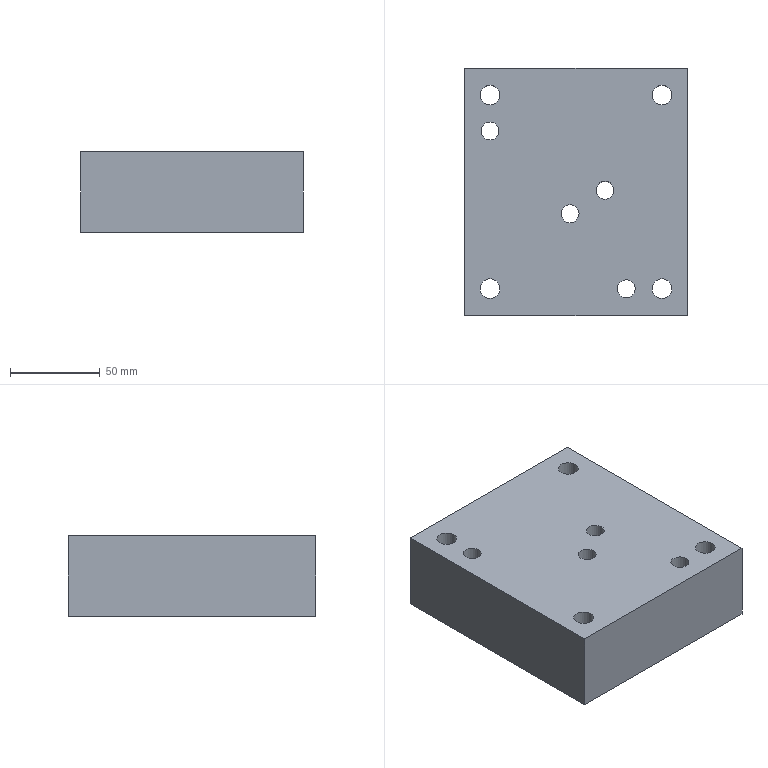Part | NX | features solid 2 | 1 solid | 32 faces | box 124 x 138 x 45 mm | volume 721952 mm3 | cylinder 17 | plane 12 | cone 3 | commonest cylinder face diameters 10 x4 11 x4 17 x4 8.5 x3 12 x2
STEP:
#1=CARTESIAN_POINT('',(391.63,-102.164,63.));
#2=VERTEX_POINT('',#1);
#3=CARTESIAN_POINT('',(397.13,-102.164,63.));
#4=DIRECTION('',(0.,0.,1.));
#5=DIRECTION('',(-1.,0.,0.));
#6=AXIS2_PLACEMENT_3D('',#3,#4,#5);
#7=CIRCLE('',#6,5.5);
#8=EDGE_CURVE('',#2,#2,#7,.T.);
#9=ORIENTED_EDGE('',*,*,#8,.T.);
#10=EDGE_LOOP('',(#9));
#11=FACE_BOUND('',#10,.T.);
#12=CARTESIAN_POINT('',(388.63,-102.164,63.));
#13=VERTEX_POINT('',#12);
#14=CARTESIAN_POINT('',(397.13,-102.164,63.));
#15=DIRECTION('',(0.,0.,1.));
#16=DIRECTION('',(-1.,0.,0.));
#17=AXIS2_PLACEMENT_3D('',#14,#15,#16);
#18=CIRCLE('',#17,8.5);
#19=EDGE_CURVE('',#13,#13,#18,.T.);
#20=ORIENTED_EDGE('',*,*,#19,.F.);
#21=EDGE_LOOP('',(#20));
#22=FACE_BOUND('',#21,.T.);
#23=CARTESIAN_POINT('',(188.,0.,63.));
#24=DIRECTION('',(0.,0.,-1.));
#25=DIRECTION('',(-1.,0.,0.));
#26=AXIS2_PLACEMENT_3D('',#23,#24,#25);
#27=PLANE('',#26);
#28=ADVANCED_FACE('',(#11,#22),#27,.T.);
#29=CARTESIAN_POINT('',(498.63,-102.164,63.));
#30=VERTEX_POINT('',#29);
#31=CARTESIAN_POINT('',(493.13,-102.164,63.));
#32=DIRECTION('',(0.,0.,-1.));
#33=DIRECTION('',(1.,0.,0.));
#34=AXIS2_PLACEMENT_3D('',#31,#32,#33);
#35=CIRCLE('',#34,5.5);
#36=EDGE_CURVE('',#30,#30,#35,.F.);
#37=ORIENTED_EDGE('',*,*,#36,.T.);
#38=EDGE_LOOP('',(#37));
#39=FACE_BOUND('',#38,.T.);
#40=CARTESIAN_POINT('',(501.63,-102.164,63.));
#41=VERTEX_POINT('',#40);
#42=CARTESIAN_POINT('',(493.13,-102.164,63.));
#43=DIRECTION('',(0.,0.,-1.));
#44=DIRECTION('',(1.,0.,0.));
#45=AXIS2_PLACEMENT_3D('',#42,#43,#44);
#46=CIRCLE('',#45,8.5);
#47=EDGE_CURVE('',#41,#41,#46,.F.);
#48=ORIENTED_EDGE('',*,*,#47,.F.);
#49=EDGE_LOOP('',(#48));
#50=FACE_BOUND('',#49,.T.);
#51=CARTESIAN_POINT('',(702.259,0.,63.));
#52=DIRECTION('',(0.,0.,-1.));
#53=DIRECTION('',(1.,0.,0.));
#54=AXIS2_PLACEMENT_3D('',#51,#52,#53);
#55=PLANE('',#54);
#56=ADVANCED_FACE('',(#39,#50),#55,.T.);
#57=CARTESIAN_POINT('',(498.63,-210.164,63.));
#58=VERTEX_POINT('',#57);
#59=CARTESIAN_POINT('',(493.13,-210.164,63.));
#60=DIRECTION('',(0.,0.,1.));
#61=DIRECTION('',(1.,0.,0.));
#62=AXIS2_PLACEMENT_3D('',#59,#60,#61);
#63=CIRCLE('',#62,5.5);
#64=EDGE_CURVE('',#58,#58,#63,.T.);
#65=ORIENTED_EDGE('',*,*,#64,.T.);
#66=EDGE_LOOP('',(#65));
#67=FACE_BOUND('',#66,.T.);
#68=CARTESIAN_POINT('',(501.63,-210.164,63.));
#69=VERTEX_POINT('',#68);
#70=CARTESIAN_POINT('',(493.13,-210.164,63.));
#71=DIRECTION('',(0.,0.,1.));
#72=DIRECTION('',(1.,0.,0.));
#73=AXIS2_PLACEMENT_3D('',#70,#71,#72);
#74=CIRCLE('',#73,8.5);
#75=EDGE_CURVE('',#69,#69,#74,.T.);
#76=ORIENTED_EDGE('',*,*,#75,.F.);
#77=EDGE_LOOP('',(#76));
#78=FACE_BOUND('',#77,.T.);
#79=CARTESIAN_POINT('',(702.259,-312.328,63.));
#80=DIRECTION('',(0.,0.,-1.));
#81=DIRECTION('',(1.,0.,0.));
#82=AXIS2_PLACEMENT_3D('',#79,#80,#81);
#83=PLANE('',#82);
#84=ADVANCED_FACE('',(#67,#78),#83,.T.);
#85=CARTESIAN_POINT('',(391.63,-210.164,63.));
#86=VERTEX_POINT('',#85);
#87=CARTESIAN_POINT('',(397.13,-210.164,63.));
#88=DIRECTION('',(0.,0.,-1.));
#89=DIRECTION('',(-1.,0.,0.));
#90=AXIS2_PLACEMENT_3D('',#87,#88,#89);
#91=CIRCLE('',#90,5.5);
#92=EDGE_CURVE('',#86,#86,#91,.F.);
#93=ORIENTED_EDGE('',*,*,#92,.T.);
#94=EDGE_LOOP('',(#93));
#95=FACE_BOUND('',#94,.T.);
#96=CARTESIAN_POINT('',(388.63,-210.164,63.));
#97=VERTEX_POINT('',#96);
#98=CARTESIAN_POINT('',(397.13,-210.164,63.));
#99=DIRECTION('',(0.,0.,-1.));
#100=DIRECTION('',(-1.,0.,0.));
#101=AXIS2_PLACEMENT_3D('',#98,#99,#100);
#102=CIRCLE('',#101,8.5);
#103=EDGE_CURVE('',#97,#97,#102,.F.);
#104=ORIENTED_EDGE('',*,*,#103,.F.);
#105=EDGE_LOOP('',(#104));
#106=FACE_BOUND('',#105,.T.);
#107=CARTESIAN_POINT('',(188.,-312.328,63.));
#108=DIRECTION('',(0.,0.,-1.));
#109=DIRECTION('',(-1.,0.,0.));
#110=AXIS2_PLACEMENT_3D('',#107,#108,#109);
#111=PLANE('',#110);
#112=ADVANCED_FACE('',(#95,#106),#111,.T.);
#113=CARTESIAN_POINT('',(402.13,-122.164,58.));
#114=VERTEX_POINT('',#113);
#115=CARTESIAN_POINT('',(397.13,-122.164,58.));
#116=DIRECTION('',(0.,0.,-1.));
#117=DIRECTION('',(1.,0.,0.));
#118=AXIS2_PLACEMENT_3D('',#115,#116,#117);
#119=CIRCLE('',#118,5.);
#120=EDGE_CURVE('',#114,#114,#119,.F.);
#121=ORIENTED_EDGE('',*,*,#120,.T.);
#122=EDGE_LOOP('',(#121));
#123=FACE_BOUND('',#122,.T.);
#124=CARTESIAN_POINT('',(403.13,-122.164,58.));
#125=VERTEX_POINT('',#124);
#126=CARTESIAN_POINT('',(397.13,-122.164,58.));
#127=DIRECTION('',(0.,0.,-1.));
#128=DIRECTION('',(1.,0.,0.));
#129=AXIS2_PLACEMENT_3D('',#126,#127,#128);
#130=CIRCLE('',#129,6.);
#131=EDGE_CURVE('',#125,#125,#130,.F.);
#132=ORIENTED_EDGE('',*,*,#131,.F.);
#133=EDGE_LOOP('',(#132));
#134=FACE_BOUND('',#133,.T.);
#135=CARTESIAN_POINT('',(397.575,-126.335,58.));
#136=DIRECTION('',(0.,0.,1.));
#137=DIRECTION('',(1.,0.,0.));
#138=AXIS2_PLACEMENT_3D('',#135,#136,#137);
#139=PLANE('',#138);
#140=ADVANCED_FACE('',(#123,#134),#139,.F.);
#141=CARTESIAN_POINT('',(402.13,-122.164,88.));
#142=VERTEX_POINT('',#141);
#143=CARTESIAN_POINT('',(397.13,-122.164,88.));
#144=DIRECTION('',(0.,0.,-1.));
#145=DIRECTION('',(1.,0.,0.));
#146=AXIS2_PLACEMENT_3D('',#143,#144,#145);
#147=CIRCLE('',#146,5.);
#148=EDGE_CURVE('',#142,#142,#147,.F.);
#149=ORIENTED_EDGE('',*,*,#148,.T.);
#150=EDGE_LOOP('',(#149));
#151=FACE_BOUND('',#150,.T.);
#152=ORIENTED_EDGE('',*,*,#120,.F.);
#153=EDGE_LOOP('',(#152));
#154=FACE_BOUND('',#153,.T.);
#155=CARTESIAN_POINT('',(397.13,-122.164,78.));
#156=DIRECTION('',(0.,0.,1.));
#157=DIRECTION('',(1.,0.,0.));
#158=AXIS2_PLACEMENT_3D('',#155,#156,#157);
#159=CYLINDRICAL_SURFACE('',#158,5.);
#160=ADVANCED_FACE('',(#151,#154),#159,.F.);
#161=CARTESIAN_POINT('',(402.63,-210.164,88.));
#162=VERTEX_POINT('',#161);
#163=CARTESIAN_POINT('',(397.13,-210.164,88.));
#164=DIRECTION('',(0.,0.,1.));
#165=DIRECTION('',(1.,0.,0.));
#166=AXIS2_PLACEMENT_3D('',#163,#164,#165);
#167=CIRCLE('',#166,5.5);
#168=EDGE_CURVE('',#162,#162,#167,.T.);
#169=ORIENTED_EDGE('',*,*,#168,.T.);
#170=EDGE_LOOP('',(#169));
#171=FACE_BOUND('',#170,.T.);
#172=ORIENTED_EDGE('',*,*,#92,.F.);
#173=EDGE_LOOP('',(#172));
#174=FACE_BOUND('',#173,.T.);
#175=CARTESIAN_POINT('',(397.13,-210.164,78.));
#176=DIRECTION('',(0.,0.,1.));
#177=DIRECTION('',(1.,0.,0.));
#178=AXIS2_PLACEMENT_3D('',#175,#176,#177);
#179=CYLINDRICAL_SURFACE('',#178,5.5);
#180=ADVANCED_FACE('',(#171,#174),#179,.F.);
#181=CARTESIAN_POINT('',(487.63,-210.164,88.));
#182=VERTEX_POINT('',#181);
#183=CARTESIAN_POINT('',(493.13,-210.164,88.));
#184=DIRECTION('',(0.,0.,-1.));
#185=DIRECTION('',(-1.,0.,0.));
#186=AXIS2_PLACEMENT_3D('',#183,#184,#185);
#187=CIRCLE('',#186,5.5);
#188=EDGE_CURVE('',#182,#182,#187,.F.);
#189=ORIENTED_EDGE('',*,*,#188,.T.);
#190=EDGE_LOOP('',(#189));
#191=FACE_BOUND('',#190,.T.);
#192=ORIENTED_EDGE('',*,*,#64,.F.);
#193=EDGE_LOOP('',(#192));
#194=FACE_BOUND('',#193,.T.);
#195=CARTESIAN_POINT('',(493.13,-210.164,78.));
#196=DIRECTION('',(0.,0.,1.));
#197=DIRECTION('',(-1.,0.,0.));
#198=AXIS2_PLACEMENT_3D('',#195,#196,#197);
#199=CYLINDRICAL_SURFACE('',#198,5.5);
#200=ADVANCED_FACE('',(#191,#194),#199,.F.);
#201=CARTESIAN_POINT('',(487.63,-102.164,88.));
#202=VERTEX_POINT('',#201);
#203=CARTESIAN_POINT('',(493.13,-102.164,88.));
#204=DIRECTION('',(0.,0.,1.));
#205=DIRECTION('',(-1.,0.,0.));
#206=AXIS2_PLACEMENT_3D('',#203,#204,#205);
#207=CIRCLE('',#206,5.5);
#208=EDGE_CURVE('',#202,#202,#207,.T.);
#209=ORIENTED_EDGE('',*,*,#208,.T.);
#210=EDGE_LOOP('',(#209));
#211=FACE_BOUND('',#210,.T.);
#212=ORIENTED_EDGE('',*,*,#36,.F.);
#213=EDGE_LOOP('',(#212));
#214=FACE_BOUND('',#213,.T.);
#215=CARTESIAN_POINT('',(493.13,-102.164,78.));
#216=DIRECTION('',(0.,0.,1.));
#217=DIRECTION('',(-1.,0.,0.));
#218=AXIS2_PLACEMENT_3D('',#215,#216,#217);
#219=CYLINDRICAL_SURFACE('',#218,5.5);
#220=ADVANCED_FACE('',(#211,#214),#219,.F.);
#221=CARTESIAN_POINT('',(383.13,-225.164,43.));
#222=VERTEX_POINT('',#221);
#223=CARTESIAN_POINT('',(383.13,-225.164,88.));
#224=VERTEX_POINT('',#223);
#225=CARTESIAN_POINT('',(383.13,-225.164,62.));
#226=DIRECTION('',(0.,0.,1.));
#227=VECTOR('',#226,1000.);
#228=LINE('',#225,#227);
#229=EDGE_CURVE('',#222,#224,#228,.T.);
#230=ORIENTED_EDGE('',*,*,#229,.F.);
#231=CARTESIAN_POINT('',(507.13,-225.164,43.));
#232=VERTEX_POINT('',#231);
#233=CARTESIAN_POINT('',(445.13,-225.164,43.));
#234=DIRECTION('',(-1.,0.,0.));
#235=VECTOR('',#234,1000.);
#236=LINE('',#233,#235);
#237=EDGE_CURVE('',#232,#222,#236,.T.);
#238=ORIENTED_EDGE('',*,*,#237,.F.);
#239=CARTESIAN_POINT('',(507.13,-225.164,88.));
#240=VERTEX_POINT('',#239);
#241=CARTESIAN_POINT('',(507.13,-225.164,62.));
#242=DIRECTION('',(0.,0.,1.));
#243=VECTOR('',#242,1000.);
#244=LINE('',#241,#243);
#245=EDGE_CURVE('',#232,#240,#244,.T.);
#246=ORIENTED_EDGE('',*,*,#245,.T.);
#247=CARTESIAN_POINT('',(445.13,-225.164,88.));
#248=DIRECTION('',(1.,0.,0.));
#249=VECTOR('',#248,1000.);
#250=LINE('',#247,#249);
#251=EDGE_CURVE('',#224,#240,#250,.T.);
#252=ORIENTED_EDGE('',*,*,#251,.F.);
#253=EDGE_LOOP('',(#230,#238,#246,#252));
#254=FACE_BOUND('',#253,.T.);
#255=CARTESIAN_POINT('',(445.13,-225.164,62.));
#256=DIRECTION('',(0.,-1.,0.));
#257=DIRECTION('',(0.,0.,1.));
#258=AXIS2_PLACEMENT_3D('',#255,#256,#257);
#259=PLANE('',#258);
#260=ADVANCED_FACE('',(#254),#259,.T.);
#261=CARTESIAN_POINT('',(383.13,-87.164,43.));
#262=VERTEX_POINT('',#261);
#263=CARTESIAN_POINT('',(383.13,-87.164,88.));
#264=VERTEX_POINT('',#263);
#265=CARTESIAN_POINT('',(383.13,-87.164,62.));
#266=DIRECTION('',(0.,0.,1.));
#267=VECTOR('',#266,1000.);
#268=LINE('',#265,#267);
#269=EDGE_CURVE('',#262,#264,#268,.T.);
#270=ORIENTED_EDGE('',*,*,#269,.F.);
#271=CARTESIAN_POINT('',(383.13,-154.023,43.));
#272=DIRECTION('',(0.,1.,0.));
#273=VECTOR('',#272,1000.);
#274=LINE('',#271,#273);
#275=EDGE_CURVE('',#222,#262,#274,.T.);
#276=ORIENTED_EDGE('',*,*,#275,.F.);
#277=ORIENTED_EDGE('',*,*,#229,.T.);
#278=CARTESIAN_POINT('',(383.13,-154.023,88.));
#279=DIRECTION('',(0.,-1.,0.));
#280=VECTOR('',#279,1000.);
#281=LINE('',#278,#280);
#282=EDGE_CURVE('',#264,#224,#281,.T.);
#283=ORIENTED_EDGE('',*,*,#282,.F.);
#284=EDGE_LOOP('',(#270,#276,#277,#283));
#285=FACE_BOUND('',#284,.T.);
#286=CARTESIAN_POINT('',(383.13,-154.023,62.));
#287=DIRECTION('',(-1.,0.,0.));
#288=DIRECTION('',(0.,0.,1.));
#289=AXIS2_PLACEMENT_3D('',#286,#287,#288);
#290=PLANE('',#289);
#291=ADVANCED_FACE('',(#285),#290,.T.);
#292=CARTESIAN_POINT('',(507.13,-87.164,43.));
#293=VERTEX_POINT('',#292);
#294=CARTESIAN_POINT('',(507.13,-87.164,88.));
#295=VERTEX_POINT('',#294);
#296=CARTESIAN_POINT('',(507.13,-87.164,62.));
#297=DIRECTION('',(0.,0.,1.));
#298=VECTOR('',#297,1000.);
#299=LINE('',#296,#298);
#300=EDGE_CURVE('',#293,#295,#299,.T.);
#301=ORIENTED_EDGE('',*,*,#300,.F.);
#302=CARTESIAN_POINT('',(445.13,-87.164,43.));
#303=DIRECTION('',(1.,0.,0.));
#304=VECTOR('',#303,1000.);
#305=LINE('',#302,#304);
#306=EDGE_CURVE('',#262,#293,#305,.T.);
#307=ORIENTED_EDGE('',*,*,#306,.F.);
#308=ORIENTED_EDGE('',*,*,#269,.T.);
#309=CARTESIAN_POINT('',(445.13,-87.164,88.));
#310=DIRECTION('',(-1.,0.,0.));
#311=VECTOR('',#310,1000.);
#312=LINE('',#309,#311);
#313=EDGE_CURVE('',#295,#264,#312,.T.);
#314=ORIENTED_EDGE('',*,*,#313,.F.);
#315=EDGE_LOOP('',(#301,#307,#308,#314));
#316=FACE_BOUND('',#315,.T.);
#317=CARTESIAN_POINT('',(445.13,-87.164,62.));
#318=DIRECTION('',(0.,1.,0.));
#319=DIRECTION('',(0.,0.,-1.));
#320=AXIS2_PLACEMENT_3D('',#317,#318,#319);
#321=PLANE('',#320);
#322=ADVANCED_FACE('',(#316),#321,.T.);
#323=CARTESIAN_POINT('',(507.13,-154.023,43.));
#324=DIRECTION('',(0.,-1.,0.));
#325=VECTOR('',#324,1000.);
#326=LINE('',#323,#325);
#327=EDGE_CURVE('',#293,#232,#326,.T.);
#328=ORIENTED_EDGE('',*,*,#327,.F.);
#329=ORIENTED_EDGE('',*,*,#300,.T.);
#330=CARTESIAN_POINT('',(507.13,-154.023,88.));
#331=DIRECTION('',(0.,1.,0.));
#332=VECTOR('',#331,1000.);
#333=LINE('',#330,#332);
#334=EDGE_CURVE('',#240,#295,#333,.T.);
#335=ORIENTED_EDGE('',*,*,#334,.F.);
#336=ORIENTED_EDGE('',*,*,#245,.F.);
#337=EDGE_LOOP('',(#328,#329,#335,#336));
#338=FACE_BOUND('',#337,.T.);
#339=CARTESIAN_POINT('',(507.13,-154.023,62.));
#340=DIRECTION('',(1.,0.,0.));
#341=DIRECTION('',(0.,0.,-1.));
#342=AXIS2_PLACEMENT_3D('',#339,#340,#341);
#343=PLANE('',#342);
#344=ADVANCED_FACE('',(#338),#343,.T.);
#345=ORIENTED_EDGE('',*,*,#19,.T.);
#346=EDGE_LOOP('',(#345));
#347=FACE_BOUND('',#346,.T.);
#348=CARTESIAN_POINT('',(405.63,-102.164,43.));
#349=VERTEX_POINT('',#348);
#350=CARTESIAN_POINT('',(397.13,-102.164,43.));
#351=DIRECTION('',(0.,0.,-1.));
#352=DIRECTION('',(1.,0.,0.));
#353=AXIS2_PLACEMENT_3D('',#350,#351,#352);
#354=CIRCLE('',#353,8.5);
#355=EDGE_CURVE('',#349,#349,#354,.T.);
#356=ORIENTED_EDGE('',*,*,#355,.T.);
#357=EDGE_LOOP('',(#356));
#358=FACE_BOUND('',#357,.T.);
#359=CARTESIAN_POINT('',(397.13,-102.164,43.));
#360=DIRECTION('',(0.,0.,1.));
#361=DIRECTION('',(1.,0.,0.));
#362=AXIS2_PLACEMENT_3D('',#359,#360,#361);
#363=CYLINDRICAL_SURFACE('',#362,8.5);
#364=ADVANCED_FACE('',(#347,#358),#363,.F.);
#365=ORIENTED_EDGE('',*,*,#47,.T.);
#366=EDGE_LOOP('',(#365));
#367=FACE_BOUND('',#366,.T.);
#368=CARTESIAN_POINT('',(484.63,-102.164,43.));
#369=VERTEX_POINT('',#368);
#370=CARTESIAN_POINT('',(493.13,-102.164,43.));
#371=DIRECTION('',(0.,0.,1.));
#372=DIRECTION('',(-1.,0.,0.));
#373=AXIS2_PLACEMENT_3D('',#370,#371,#372);
#374=CIRCLE('',#373,8.5);
#375=EDGE_CURVE('',#369,#369,#374,.F.);
#376=ORIENTED_EDGE('',*,*,#375,.T.);
#377=EDGE_LOOP('',(#376));
#378=FACE_BOUND('',#377,.T.);
#379=CARTESIAN_POINT('',(493.13,-102.164,43.));
#380=DIRECTION('',(0.,0.,1.));
#381=DIRECTION('',(-1.,0.,0.));
#382=AXIS2_PLACEMENT_3D('',#379,#380,#381);
#383=CYLINDRICAL_SURFACE('',#382,8.5);
#384=ADVANCED_FACE('',(#367,#378),#383,.F.);
#385=ORIENTED_EDGE('',*,*,#75,.T.);
#386=EDGE_LOOP('',(#385));
#387=FACE_BOUND('',#386,.T.);
#388=CARTESIAN_POINT('',(484.63,-210.164,43.));
#389=VERTEX_POINT('',#388);
#390=CARTESIAN_POINT('',(493.13,-210.164,43.));
#391=DIRECTION('',(0.,0.,-1.));
#392=DIRECTION('',(-1.,0.,0.));
#393=AXIS2_PLACEMENT_3D('',#390,#391,#392);
#394=CIRCLE('',#393,8.5);
#395=EDGE_CURVE('',#389,#389,#394,.T.);
#396=ORIENTED_EDGE('',*,*,#395,.T.);
#397=EDGE_LOOP('',(#396));
#398=FACE_BOUND('',#397,.T.);
#399=CARTESIAN_POINT('',(493.13,-210.164,43.));
#400=DIRECTION('',(0.,0.,1.));
#401=DIRECTION('',(-1.,0.,0.));
#402=AXIS2_PLACEMENT_3D('',#399,#400,#401);
#403=CYLINDRICAL_SURFACE('',#402,8.5);
#404=ADVANCED_FACE('',(#387,#398),#403,.F.);
#405=ORIENTED_EDGE('',*,*,#103,.T.);
#406=EDGE_LOOP('',(#405));
#407=FACE_BOUND('',#406,.T.);
#408=CARTESIAN_POINT('',(405.63,-210.164,43.));
#409=VERTEX_POINT('',#408);
#410=CARTESIAN_POINT('',(397.13,-210.164,43.));
#411=DIRECTION('',(0.,0.,1.));
#412=DIRECTION('',(1.,0.,0.));
#413=AXIS2_PLACEMENT_3D('',#410,#411,#412);
#414=CIRCLE('',#413,8.5);
#415=EDGE_CURVE('',#409,#409,#414,.F.);
#416=ORIENTED_EDGE('',*,*,#415,.T.);
#417=EDGE_LOOP('',(#416));
#418=FACE_BOUND('',#417,.T.);
#419=CARTESIAN_POINT('',(397.13,-210.164,43.));
#420=DIRECTION('',(0.,0.,1.));
#421=DIRECTION('',(1.,0.,0.));
#422=AXIS2_PLACEMENT_3D('',#419,#420,#421);
#423=CYLINDRICAL_SURFACE('',#422,8.5);
#424=ADVANCED_FACE('',(#407,#418),#423,.F.);
#425=ORIENTED_EDGE('',*,*,#131,.T.);
#426=EDGE_LOOP('',(#425));
#427=FACE_BOUND('',#426,.T.);
#428=CARTESIAN_POINT('',(403.13,-122.164,43.));
#429=VERTEX_POINT('',#428);
#430=CARTESIAN_POINT('',(397.13,-122.164,43.));
#431=DIRECTION('',(0.,0.,-1.));
#432=DIRECTION('',(1.,0.,0.));
#433=AXIS2_PLACEMENT_3D('',#430,#431,#432);
#434=CIRCLE('',#433,6.);
#435=EDGE_CURVE('',#429,#429,#434,.T.);
#436=ORIENTED_EDGE('',*,*,#435,.T.);
#437=EDGE_LOOP('',(#436));
#438=FACE_BOUND('',#437,.T.);
#439=CARTESIAN_POINT('',(397.13,-122.164,43.));
#440=DIRECTION('',(0.,0.,1.));
#441=DIRECTION('',(1.,0.,0.));
#442=AXIS2_PLACEMENT_3D('',#439,#440,#441);
#443=CYLINDRICAL_SURFACE('',#442,6.);
#444=ADVANCED_FACE('',(#427,#438),#443,.F.);
#445=CARTESIAN_POINT('',(446.804,-168.277,43.));
#446=VERTEX_POINT('',#445);
#447=CARTESIAN_POINT('',(441.804,-168.277,43.));
#448=DIRECTION('',(0.,0.,1.));
#449=DIRECTION('',(1.,0.,0.));
#450=AXIS2_PLACEMENT_3D('',#447,#448,#449);
#451=CIRCLE('',#450,5.);
#452=EDGE_CURVE('',#446,#446,#451,.T.);
#453=ORIENTED_EDGE('',*,*,#452,.T.);
#454=EDGE_LOOP('',(#453));
#455=FACE_BOUND('',#454,.T.);
#456=CARTESIAN_POINT('',(466.304,-155.277,43.));
#457=VERTEX_POINT('',#456);
#458=CARTESIAN_POINT('',(461.304,-155.277,43.));
#459=DIRECTION('',(0.,0.,1.));
#460=DIRECTION('',(1.,0.,0.));
#461=AXIS2_PLACEMENT_3D('',#458,#459,#460);
#462=CIRCLE('',#461,5.);
#463=EDGE_CURVE('',#457,#457,#462,.T.);
#464=ORIENTED_EDGE('',*,*,#463,.T.);
#465=EDGE_LOOP('',(#464));
#466=FACE_BOUND('',#465,.T.);
#467=CARTESIAN_POINT('',(452.054,-139.208,43.));
#468=VERTEX_POINT('',#467);
#469=CARTESIAN_POINT('',(447.804,-139.208,43.));
#470=DIRECTION('',(0.,0.,1.));
#471=DIRECTION('',(1.,0.,0.));
#472=AXIS2_PLACEMENT_3D('',#469,#470,#471);
#473=CIRCLE('',#472,4.25);
#474=EDGE_CURVE('',#468,#468,#473,.T.);
#475=ORIENTED_EDGE('',*,*,#474,.T.);
#476=EDGE_LOOP('',(#475));
#477=FACE_BOUND('',#476,.T.);
#478=CARTESIAN_POINT('',(420.887,-180.642,43.));
#479=VERTEX_POINT('',#478);
#480=CARTESIAN_POINT('',(416.637,-180.642,43.));
#481=DIRECTION('',(0.,0.,1.));
#482=DIRECTION('',(1.,0.,0.));
#483=AXIS2_PLACEMENT_3D('',#480,#481,#482);
#484=CIRCLE('',#483,4.25);
#485=EDGE_CURVE('',#479,#479,#484,.T.);
#486=ORIENTED_EDGE('',*,*,#485,.T.);
#487=EDGE_LOOP('',(#486));
#488=FACE_BOUND('',#487,.T.);
#489=CARTESIAN_POINT('',(477.887,-180.642,43.));
#490=VERTEX_POINT('',#489);
#491=CARTESIAN_POINT('',(473.637,-180.642,43.));
#492=DIRECTION('',(0.,0.,1.));
#493=DIRECTION('',(1.,0.,0.));
#494=AXIS2_PLACEMENT_3D('',#491,#492,#493);
#495=CIRCLE('',#494,4.25);
#496=EDGE_CURVE('',#490,#490,#495,.T.);
#497=ORIENTED_EDGE('',*,*,#496,.T.);
#498=EDGE_LOOP('',(#497));
#499=FACE_BOUND('',#498,.T.);
#500=CARTESIAN_POINT('',(479.13,-210.164,43.));
#501=VERTEX_POINT('',#500);
#502=CARTESIAN_POINT('',(473.13,-210.164,43.));
#503=DIRECTION('',(0.,0.,-1.));
#504=DIRECTION('',(1.,0.,0.));
#505=AXIS2_PLACEMENT_3D('',#502,#503,#504);
#506=CIRCLE('',#505,6.);
#507=EDGE_CURVE('',#501,#501,#506,.F.);
#508=ORIENTED_EDGE('',*,*,#507,.T.);
#509=EDGE_LOOP('',(#508));
#510=FACE_BOUND('',#509,.T.);
#511=ORIENTED_EDGE('',*,*,#435,.F.);
#512=EDGE_LOOP('',(#511));
#513=FACE_BOUND('',#512,.T.);
#514=ORIENTED_EDGE('',*,*,#415,.F.);
#515=EDGE_LOOP('',(#514));
#516=FACE_BOUND('',#515,.T.);
#517=ORIENTED_EDGE('',*,*,#395,.F.);
#518=EDGE_LOOP('',(#517));
#519=FACE_BOUND('',#518,.T.);
#520=ORIENTED_EDGE('',*,*,#375,.F.);
#521=EDGE_LOOP('',(#520));
#522=FACE_BOUND('',#521,.T.);
#523=ORIENTED_EDGE('',*,*,#355,.F.);
#524=EDGE_LOOP('',(#523));
#525=FACE_BOUND('',#524,.T.);
#526=ORIENTED_EDGE('',*,*,#327,.T.);
#527=ORIENTED_EDGE('',*,*,#237,.T.);
#528=ORIENTED_EDGE('',*,*,#275,.T.);
#529=ORIENTED_EDGE('',*,*,#306,.T.);
#530=EDGE_LOOP('',(#526,#527,#528,#529));
#531=FACE_BOUND('',#530,.T.);
#532=CARTESIAN_POINT('',(188.,0.,43.));
#533=DIRECTION('',(0.,0.,-1.));
#534=DIRECTION('',(-1.,0.,0.));
#535=AXIS2_PLACEMENT_3D('',#532,#533,#534);
#536=PLANE('',#535);
#537=ADVANCED_FACE('',(#455,#466,#477,#488,#499,#510,#513,#516,#519,#522,#525,#531),#536,.T.);
#538=CARTESIAN_POINT('',(402.63,-102.164,88.));
#539=VERTEX_POINT('',#538);
#540=CARTESIAN_POINT('',(397.13,-102.164,88.));
#541=DIRECTION('',(0.,0.,-1.));
#542=DIRECTION('',(1.,0.,0.));
#543=AXIS2_PLACEMENT_3D('',#540,#541,#542);
#544=CIRCLE('',#543,5.5);
#545=EDGE_CURVE('',#539,#539,#544,.F.);
#546=ORIENTED_EDGE('',*,*,#545,.T.);
#547=EDGE_LOOP('',(#546));
#548=FACE_BOUND('',#547,.T.);
#549=ORIENTED_EDGE('',*,*,#8,.F.);
#550=EDGE_LOOP('',(#549));
#551=FACE_BOUND('',#550,.T.);
#552=CARTESIAN_POINT('',(397.13,-102.164,78.));
#553=DIRECTION('',(0.,0.,1.));
#554=DIRECTION('',(1.,0.,0.));
#555=AXIS2_PLACEMENT_3D('',#552,#553,#554);
#556=CYLINDRICAL_SURFACE('',#555,5.5);
#557=ADVANCED_FACE('',(#548,#551),#556,.F.);
#558=CARTESIAN_POINT('',(446.804,-168.277,88.));
#559=VERTEX_POINT('',#558);
#560=CARTESIAN_POINT('',(441.804,-168.277,88.));
#561=DIRECTION('',(0.,0.,1.));
#562=DIRECTION('',(1.,0.,0.));
#563=AXIS2_PLACEMENT_3D('',#560,#561,#562);
#564=CIRCLE('',#563,5.);
#565=EDGE_CURVE('',#559,#559,#564,.T.);
#566=ORIENTED_EDGE('',*,*,#565,.F.);
#567=EDGE_LOOP('',(#566));
#568=FACE_BOUND('',#567,.T.);
#569=CARTESIAN_POINT('',(466.304,-155.277,88.));
#570=VERTEX_POINT('',#569);
#571=CARTESIAN_POINT('',(461.304,-155.277,88.));
#572=DIRECTION('',(0.,0.,1.));
#573=DIRECTION('',(1.,0.,0.));
#574=AXIS2_PLACEMENT_3D('',#571,#572,#573);
#575=CIRCLE('',#574,5.);
#576=EDGE_CURVE('',#570,#570,#575,.T.);
#577=ORIENTED_EDGE('',*,*,#576,.F.);
#578=EDGE_LOOP('',(#577));
#579=FACE_BOUND('',#578,.T.);
#580=CARTESIAN_POINT('',(478.13,-210.164,88.));
#581=VERTEX_POINT('',#580);
#582=CARTESIAN_POINT('',(473.13,-210.164,88.));
#583=DIRECTION('',(0.,0.,-1.));
#584=DIRECTION('',(1.,0.,0.));
#585=AXIS2_PLACEMENT_3D('',#582,#583,#584);
#586=CIRCLE('',#585,5.);
#587=EDGE_CURVE('',#581,#581,#586,.T.);
#588=ORIENTED_EDGE('',*,*,#587,.T.);
#589=EDGE_LOOP('',(#588));
#590=FACE_BOUND('',#589,.T.);
#591=ORIENTED_EDGE('',*,*,#545,.F.);
#592=EDGE_LOOP('',(#591));
#593=FACE_BOUND('',#592,.T.);
#594=ORIENTED_EDGE('',*,*,#313,.T.);
#595=ORIENTED_EDGE('',*,*,#282,.T.);
#596=ORIENTED_EDGE('',*,*,#251,.T.);
#597=ORIENTED_EDGE('',*,*,#334,.T.);
#598=EDGE_LOOP('',(#594,#595,#596,#597));
#599=FACE_BOUND('',#598,.T.);
#600=ORIENTED_EDGE('',*,*,#208,.F.);
#601=EDGE_LOOP('',(#600));
#602=FACE_BOUND('',#601,.T.);
#603=ORIENTED_EDGE('',*,*,#188,.F.);
#604=EDGE_LOOP('',(#603));
#605=FACE_BOUND('',#604,.T.);
#606=ORIENTED_EDGE('',*,*,#168,.F.);
#607=EDGE_LOOP('',(#606));
#608=FACE_BOUND('',#607,.T.);
#609=ORIENTED_EDGE('',*,*,#148,.F.);
#610=EDGE_LOOP('',(#609));
#611=FACE_BOUND('',#610,.T.);
#612=CARTESIAN_POINT('',(268.879,0.,88.));
#613=DIRECTION('',(0.,0.,1.));
#614=DIRECTION('',(-1.,0.,0.));
#615=AXIS2_PLACEMENT_3D('',#612,#613,#614);
#616=PLANE('',#615);
#617=ADVANCED_FACE('',(#568,#579,#590,#593,#599,#602,#605,#608,#611),#616,.T.);
#618=CARTESIAN_POINT('',(478.13,-210.164,58.));
#619=VERTEX_POINT('',#618);
#620=CARTESIAN_POINT('',(473.13,-210.164,58.));
#621=DIRECTION('',(0.,0.,-1.));
#622=DIRECTION('',(1.,0.,0.));
#623=AXIS2_PLACEMENT_3D('',#620,#621,#622);
#624=CIRCLE('',#623,5.);
#625=EDGE_CURVE('',#619,#619,#624,.F.);
#626=ORIENTED_EDGE('',*,*,#625,.T.);
#627=EDGE_LOOP('',(#626));
#628=FACE_BOUND('',#627,.T.);
#629=CARTESIAN_POINT('',(479.13,-210.164,58.));
#630=VERTEX_POINT('',#629);
#631=CARTESIAN_POINT('',(473.13,-210.164,58.));
#632=DIRECTION('',(0.,0.,-1.));
#633=DIRECTION('',(1.,0.,0.));
#634=AXIS2_PLACEMENT_3D('',#631,#632,#633);
#635=CIRCLE('',#634,6.);
#636=EDGE_CURVE('',#630,#630,#635,.F.);
#637=ORIENTED_EDGE('',*,*,#636,.F.);
#638=EDGE_LOOP('',(#637));
#639=FACE_BOUND('',#638,.T.);
#640=CARTESIAN_POINT('',(470.132,-216.921,58.));
#641=DIRECTION('',(0.,0.,1.));
#642=DIRECTION('',(1.,0.,0.));
#643=AXIS2_PLACEMENT_3D('',#640,#641,#642);
#644=PLANE('',#643);
#645=ADVANCED_FACE('',(#628,#639),#644,.F.);
#646=ORIENTED_EDGE('',*,*,#636,.T.);
#647=EDGE_LOOP('',(#646));
#648=FACE_BOUND('',#647,.T.);
#649=ORIENTED_EDGE('',*,*,#507,.F.);
#650=EDGE_LOOP('',(#649));
#651=FACE_BOUND('',#650,.T.);
#652=CARTESIAN_POINT('',(473.13,-210.164,43.));
#653=DIRECTION('',(0.,0.,1.));
#654=DIRECTION('',(1.,0.,0.));
#655=AXIS2_PLACEMENT_3D('',#652,#653,#654);
#656=CYLINDRICAL_SURFACE('',#655,6.);
#657=ADVANCED_FACE('',(#648,#651),#656,.F.);
#658=ORIENTED_EDGE('',*,*,#587,.F.);
#659=EDGE_LOOP('',(#658));
#660=FACE_BOUND('',#659,.T.);
#661=ORIENTED_EDGE('',*,*,#625,.F.);
#662=EDGE_LOOP('',(#661));
#663=FACE_BOUND('',#662,.T.);
#664=CARTESIAN_POINT('',(473.13,-210.164,78.));
#665=DIRECTION('',(0.,0.,1.));
#666=DIRECTION('',(1.,0.,0.));
#667=AXIS2_PLACEMENT_3D('',#664,#665,#666);
#668=CYLINDRICAL_SURFACE('',#667,5.);
#669=ADVANCED_FACE('',(#660,#663),#668,.F.);
#670=CARTESIAN_POINT('',(477.887,-180.642,73.));
#671=VERTEX_POINT('',#670);
#672=CARTESIAN_POINT('',(473.637,-180.642,73.));
#673=DIRECTION('',(0.,0.,1.));
#674=DIRECTION('',(1.,0.,0.));
#675=AXIS2_PLACEMENT_3D('',#672,#673,#674);
#676=CIRCLE('',#675,4.25);
#677=EDGE_CURVE('',#671,#671,#676,.F.);
#678=ORIENTED_EDGE('',*,*,#677,.T.);
#679=EDGE_LOOP('',(#678));
#680=FACE_BOUND('',#679,.T.);
#681=CARTESIAN_POINT('',(473.637,-180.642,75.554));
#682=VERTEX_POINT('',#681);
#683=VERTEX_LOOP('',#682);
#684=FACE_BOUND('',#683,.T.);
#685=CARTESIAN_POINT('',(473.637,-180.642,73.));
#686=DIRECTION('',(0.,0.,-1.));
#687=DIRECTION('',(-1.,0.,0.));
#688=AXIS2_PLACEMENT_3D('',#685,#686,#687);
#689=CONICAL_SURFACE('',#688,4.25,1.03);
#690=ADVANCED_FACE('',(#680,#684),#689,.F.);
#691=ORIENTED_EDGE('',*,*,#677,.F.);
#692=EDGE_LOOP('',(#691));
#693=FACE_BOUND('',#692,.T.);
#694=ORIENTED_EDGE('',*,*,#496,.F.);
#695=EDGE_LOOP('',(#694));
#696=FACE_BOUND('',#695,.T.);
#697=CARTESIAN_POINT('',(473.637,-180.642,43.));
#698=DIRECTION('',(0.,0.,1.));
#699=DIRECTION('',(1.,0.,0.));
#700=AXIS2_PLACEMENT_3D('',#697,#698,#699);
#701=CYLINDRICAL_SURFACE('',#700,4.25);
#702=ADVANCED_FACE('',(#693,#696),#701,.F.);
#703=CARTESIAN_POINT('',(420.887,-180.642,73.));
#704=VERTEX_POINT('',#703);
#705=CARTESIAN_POINT('',(416.637,-180.642,73.));
#706=DIRECTION('',(0.,0.,1.));
#707=DIRECTION('',(1.,0.,0.));
#708=AXIS2_PLACEMENT_3D('',#705,#706,#707);
#709=CIRCLE('',#708,4.25);
#710=EDGE_CURVE('',#704,#704,#709,.F.);
#711=ORIENTED_EDGE('',*,*,#710,.T.);
#712=EDGE_LOOP('',(#711));
#713=FACE_BOUND('',#712,.T.);
#714=CARTESIAN_POINT('',(416.637,-180.642,75.554));
#715=VERTEX_POINT('',#714);
#716=VERTEX_LOOP('',#715);
#717=FACE_BOUND('',#716,.T.);
#718=CARTESIAN_POINT('',(416.637,-180.642,73.));
#719=DIRECTION('',(0.,0.,-1.));
#720=DIRECTION('',(-1.,0.,0.));
#721=AXIS2_PLACEMENT_3D('',#718,#719,#720);
#722=CONICAL_SURFACE('',#721,4.25,1.03);
#723=ADVANCED_FACE('',(#713,#717),#722,.F.);
#724=ORIENTED_EDGE('',*,*,#710,.F.);
#725=EDGE_LOOP('',(#724));
#726=FACE_BOUND('',#725,.T.);
#727=ORIENTED_EDGE('',*,*,#485,.F.);
#728=EDGE_LOOP('',(#727));
#729=FACE_BOUND('',#728,.T.);
#730=CARTESIAN_POINT('',(416.637,-180.642,43.));
#731=DIRECTION('',(0.,0.,1.));
#732=DIRECTION('',(1.,0.,0.));
#733=AXIS2_PLACEMENT_3D('',#730,#731,#732);
#734=CYLINDRICAL_SURFACE('',#733,4.25);
#735=ADVANCED_FACE('',(#726,#729),#734,.F.);
#736=CARTESIAN_POINT('',(452.054,-139.208,73.));
#737=VERTEX_POINT('',#736);
#738=CARTESIAN_POINT('',(447.804,-139.208,73.));
#739=DIRECTION('',(0.,0.,1.));
#740=DIRECTION('',(1.,0.,0.));
#741=AXIS2_PLACEMENT_3D('',#738,#739,#740);
#742=CIRCLE('',#741,4.25);
#743=EDGE_CURVE('',#737,#737,#742,.F.);
#744=ORIENTED_EDGE('',*,*,#743,.T.);
#745=EDGE_LOOP('',(#744));
#746=FACE_BOUND('',#745,.T.);
#747=CARTESIAN_POINT('',(447.804,-139.208,75.554));
#748=VERTEX_POINT('',#747);
#749=VERTEX_LOOP('',#748);
#750=FACE_BOUND('',#749,.T.);
#751=CARTESIAN_POINT('',(447.804,-139.208,73.));
#752=DIRECTION('',(0.,0.,-1.));
#753=DIRECTION('',(-1.,0.,0.));
#754=AXIS2_PLACEMENT_3D('',#751,#752,#753);
#755=CONICAL_SURFACE('',#754,4.25,1.03);
#756=ADVANCED_FACE('',(#746,#750),#755,.F.);
#757=ORIENTED_EDGE('',*,*,#743,.F.);
#758=EDGE_LOOP('',(#757));
#759=FACE_BOUND('',#758,.T.);
#760=ORIENTED_EDGE('',*,*,#474,.F.);
#761=EDGE_LOOP('',(#760));
#762=FACE_BOUND('',#761,.T.);
#763=CARTESIAN_POINT('',(447.804,-139.208,43.));
#764=DIRECTION('',(0.,0.,1.));
#765=DIRECTION('',(1.,0.,0.));
#766=AXIS2_PLACEMENT_3D('',#763,#764,#765);
#767=CYLINDRICAL_SURFACE('',#766,4.25);
#768=ADVANCED_FACE('',(#759,#762),#767,.F.);
#769=ORIENTED_EDGE('',*,*,#576,.T.);
#770=EDGE_LOOP('',(#769));
#771=FACE_BOUND('',#770,.T.);
#772=ORIENTED_EDGE('',*,*,#463,.F.);
#773=EDGE_LOOP('',(#772));
#774=FACE_BOUND('',#773,.T.);
#775=CARTESIAN_POINT('',(461.304,-155.277,43.));
#776=DIRECTION('',(0.,0.,1.));
#777=DIRECTION('',(1.,0.,0.));
#778=AXIS2_PLACEMENT_3D('',#775,#776,#777);
#779=CYLINDRICAL_SURFACE('',#778,5.);
#780=ADVANCED_FACE('',(#771,#774),#779,.F.);
#781=ORIENTED_EDGE('',*,*,#565,.T.);
#782=EDGE_LOOP('',(#781));
#783=FACE_BOUND('',#782,.T.);
#784=ORIENTED_EDGE('',*,*,#452,.F.);
#785=EDGE_LOOP('',(#784));
#786=FACE_BOUND('',#785,.T.);
#787=CARTESIAN_POINT('',(441.804,-168.277,43.));
#788=DIRECTION('',(0.,0.,1.));
#789=DIRECTION('',(1.,0.,0.));
#790=AXIS2_PLACEMENT_3D('',#787,#788,#789);
#791=CYLINDRICAL_SURFACE('',#790,5.);
#792=ADVANCED_FACE('',(#783,#786),#791,.F.);
#793=CLOSED_SHELL('',(#28,#56,#84,#112,#140,#160,#180,#200,#220,#260,#291,#322,#344,#364,#384,#404,#424,#444,#537,#557,#617,#645,#657,#669,#690,#702,#723,#735,#756,#768,#780,#792));
#794=MANIFOLD_SOLID_BREP('',#793);
#795=(LENGTH_UNIT()NAMED_UNIT(*)SI_UNIT(.MILLI.,.METRE.));
#796=UNCERTAINTY_MEASURE_WITH_UNIT(LENGTH_MEASURE(0.00001),#795,'','');
#797=(NAMED_UNIT(*)PLANE_ANGLE_UNIT()SI_UNIT($,.RADIAN.));
#798=(NAMED_UNIT(*)SI_UNIT($,.STERADIAN.)SOLID_ANGLE_UNIT());
#799=(GEOMETRIC_REPRESENTATION_CONTEXT(3)GLOBAL_UNCERTAINTY_ASSIGNED_CONTEXT((#796))GLOBAL_UNIT_ASSIGNED_CONTEXT((#795,#797,#798))REPRESENTATION_CONTEXT('',''));
#800=ADVANCED_BREP_SHAPE_REPRESENTATION('',(#794),#799);